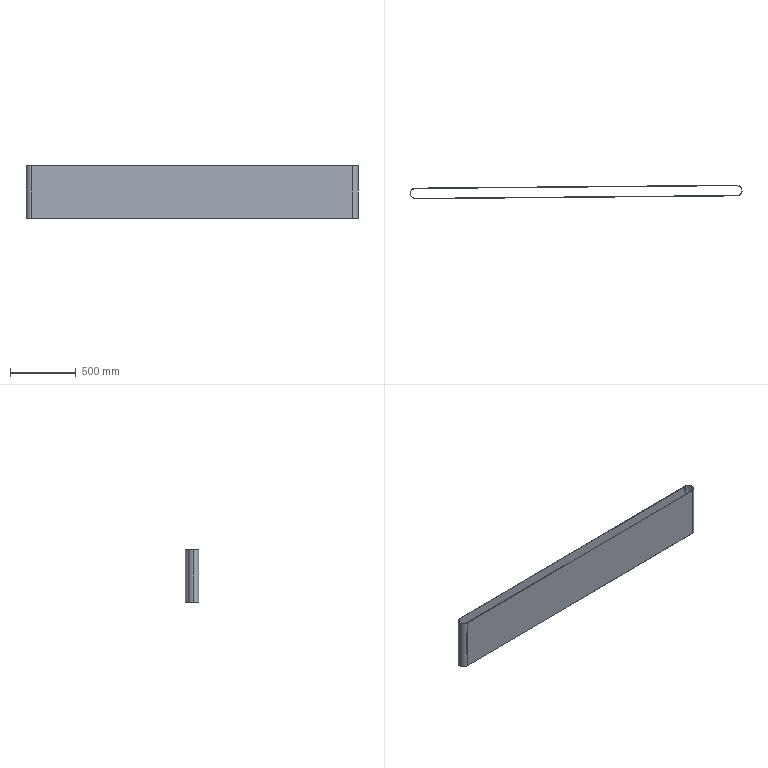Part | STEP file | Flat conveyor mechanism-strip | 1 solid | 18 faces | box 2534 x 103.36 x 400 mm | volume 5769946 mm3 | plane 12 | cylinder 6 | commonest cylinder face diameters 75.388 x3 80.988 x3
STEP:
#1=CARTESIAN_POINT('',(-1278.165,-120.803,200.));
#2=VERTEX_POINT('',#1);
#3=CARTESIAN_POINT('',(-1240.815,-83.11,200.));
#4=VERTEX_POINT('',#3);
#5=CARTESIAN_POINT('',(-1240.471,-120.803,200.));
#6=DIRECTION('',(0.,0.,-1.));
#7=DIRECTION('',(0.00912,-1.,0.));
#8=AXIS2_PLACEMENT_3D('',#5,#6,#7);
#9=CIRCLE('',#8,37.694);
#10=EDGE_CURVE('',#2,#4,#9,.T.);
#11=ORIENTED_EDGE('',*,*,#10,.F.);
#12=CARTESIAN_POINT('',(-1278.165,-120.803,-200.));
#13=VERTEX_POINT('',#12);
#14=CARTESIAN_POINT('',(-1278.165,-120.803,0.));
#15=DIRECTION('',(0.,0.,-1.));
#16=VECTOR('',#15,1000.);
#17=LINE('',#14,#16);
#18=EDGE_CURVE('',#2,#13,#17,.T.);
#19=ORIENTED_EDGE('',*,*,#18,.T.);
#20=CARTESIAN_POINT('',(-1240.815,-83.11,-200.));
#21=VERTEX_POINT('',#20);
#22=CARTESIAN_POINT('',(-1240.471,-120.803,-200.));
#23=DIRECTION('',(0.,0.,-1.));
#24=DIRECTION('',(0.00912,-1.,0.));
#25=AXIS2_PLACEMENT_3D('',#22,#23,#24);
#26=CIRCLE('',#25,37.694);
#27=EDGE_CURVE('',#13,#21,#26,.T.);
#28=ORIENTED_EDGE('',*,*,#27,.T.);
#29=CARTESIAN_POINT('',(-1240.815,-83.11,200.));
#30=DIRECTION('',(0.,0.,-1.));
#31=VECTOR('',#30,1000.);
#32=LINE('',#29,#31);
#33=EDGE_CURVE('',#4,#21,#32,.T.);
#34=ORIENTED_EDGE('',*,*,#33,.F.);
#35=EDGE_LOOP('',(#11,#19,#28,#34));
#36=FACE_OUTER_BOUND('',#35,.T.);
#37=CARTESIAN_POINT('',(-1240.471,-120.803,0.));
#38=DIRECTION('',(0.,0.,-1.));
#39=DIRECTION('',(-1.,0.,0.));
#40=AXIS2_PLACEMENT_3D('',#37,#38,#39);
#41=CYLINDRICAL_SURFACE('',#40,37.694);
#42=ADVANCED_FACE('',(#36),#41,.F.);
#43=CARTESIAN_POINT('',(-1240.101,-161.295,200.));
#44=VERTEX_POINT('',#43);
#45=CARTESIAN_POINT('',(-1280.965,-120.803,200.));
#46=VERTEX_POINT('',#45);
#47=CARTESIAN_POINT('',(-1240.471,-120.803,200.));
#48=DIRECTION('',(0.,0.,-1.));
#49=DIRECTION('',(0.00912,-1.,0.));
#50=AXIS2_PLACEMENT_3D('',#47,#48,#49);
#51=CIRCLE('',#50,40.494);
#52=EDGE_CURVE('',#44,#46,#51,.T.);
#53=ORIENTED_EDGE('',*,*,#52,.T.);
#54=CARTESIAN_POINT('',(-1280.965,-120.803,-200.));
#55=VERTEX_POINT('',#54);
#56=CARTESIAN_POINT('',(-1280.965,-120.803,0.));
#57=DIRECTION('',(0.,0.,-1.));
#58=VECTOR('',#57,1000.);
#59=LINE('',#56,#58);
#60=EDGE_CURVE('',#46,#55,#59,.T.);
#61=ORIENTED_EDGE('',*,*,#60,.T.);
#62=CARTESIAN_POINT('',(-1240.101,-161.295,-200.));
#63=VERTEX_POINT('',#62);
#64=CARTESIAN_POINT('',(-1240.471,-120.803,-200.));
#65=DIRECTION('',(0.,0.,-1.));
#66=DIRECTION('',(0.00912,-1.,0.));
#67=AXIS2_PLACEMENT_3D('',#64,#65,#66);
#68=CIRCLE('',#67,40.494);
#69=EDGE_CURVE('',#63,#55,#68,.T.);
#70=ORIENTED_EDGE('',*,*,#69,.F.);
#71=CARTESIAN_POINT('',(-1240.101,-161.295,200.));
#72=DIRECTION('',(0.,0.,1.));
#73=VECTOR('',#72,1000.);
#74=LINE('',#71,#73);
#75=EDGE_CURVE('',#63,#44,#74,.T.);
#76=ORIENTED_EDGE('',*,*,#75,.T.);
#77=EDGE_LOOP('',(#53,#61,#70,#76));
#78=FACE_OUTER_BOUND('',#77,.T.);
#79=CARTESIAN_POINT('',(-1240.471,-120.803,0.));
#80=DIRECTION('',(0.,0.,-1.));
#81=DIRECTION('',(-1.,0.,0.));
#82=AXIS2_PLACEMENT_3D('',#79,#80,#81);
#83=CYLINDRICAL_SURFACE('',#82,40.494);
#84=ADVANCED_FACE('',(#78),#83,.T.);
#85=CARTESIAN_POINT('',(-1240.84,-80.311,-200.));
#86=VERTEX_POINT('',#85);
#87=CARTESIAN_POINT('',(1212.109,-57.938,-200.));
#88=VERTEX_POINT('',#87);
#89=CARTESIAN_POINT('',(-1240.84,-80.311,-200.));
#90=DIRECTION('',(1.,0.00912,0.));
#91=VECTOR('',#90,1000.);
#92=LINE('',#89,#91);
#93=EDGE_CURVE('',#86,#88,#92,.T.);
#94=ORIENTED_EDGE('',*,*,#93,.F.);
#95=CARTESIAN_POINT('',(-1240.84,-80.311,200.));
#96=VERTEX_POINT('',#95);
#97=CARTESIAN_POINT('',(-1240.84,-80.311,200.));
#98=DIRECTION('',(0.,0.,1.));
#99=VECTOR('',#98,1000.);
#100=LINE('',#97,#99);
#101=EDGE_CURVE('',#86,#96,#100,.T.);
#102=ORIENTED_EDGE('',*,*,#101,.T.);
#103=CARTESIAN_POINT('',(1212.109,-57.938,200.));
#104=VERTEX_POINT('',#103);
#105=CARTESIAN_POINT('',(-1240.84,-80.311,200.));
#106=DIRECTION('',(1.,0.00912,0.));
#107=VECTOR('',#106,1000.);
#108=LINE('',#105,#107);
#109=EDGE_CURVE('',#96,#104,#108,.T.);
#110=ORIENTED_EDGE('',*,*,#109,.T.);
#111=CARTESIAN_POINT('',(1212.109,-57.938,200.));
#112=DIRECTION('',(0.,0.,1.));
#113=VECTOR('',#112,1000.);
#114=LINE('',#111,#113);
#115=EDGE_CURVE('',#88,#104,#114,.T.);
#116=ORIENTED_EDGE('',*,*,#115,.F.);
#117=EDGE_LOOP('',(#94,#102,#110,#116));
#118=FACE_OUTER_BOUND('',#117,.T.);
#119=CARTESIAN_POINT('',(-1240.84,-80.311,200.));
#120=DIRECTION('',(-0.00912,1.,0.));
#121=DIRECTION('',(-1.,-0.00912,0.));
#122=AXIS2_PLACEMENT_3D('',#119,#120,#121);
#123=PLANE('',#122);
#124=ADVANCED_FACE('',(#118),#123,.T.);
#125=CARTESIAN_POINT('',(1212.134,-60.738,-200.));
#126=VERTEX_POINT('',#125);
#127=CARTESIAN_POINT('',(-1240.815,-83.11,-200.));
#128=DIRECTION('',(1.,0.00912,0.));
#129=VECTOR('',#128,1000.);
#130=LINE('',#127,#129);
#131=EDGE_CURVE('',#21,#126,#130,.T.);
#132=ORIENTED_EDGE('',*,*,#131,.F.);
#133=CARTESIAN_POINT('',(-1240.84,-80.311,-200.));
#134=DIRECTION('',(-0.00912,1.,0.));
#135=VECTOR('',#134,1000.);
#136=LINE('',#133,#135);
#137=EDGE_CURVE('',#21,#86,#136,.T.);
#138=ORIENTED_EDGE('',*,*,#137,.T.);
#139=ORIENTED_EDGE('',*,*,#93,.T.);
#140=CARTESIAN_POINT('',(1212.109,-57.938,-200.));
#141=DIRECTION('',(-0.00912,1.,0.));
#142=VECTOR('',#141,1000.);
#143=LINE('',#140,#142);
#144=EDGE_CURVE('',#126,#88,#143,.T.);
#145=ORIENTED_EDGE('',*,*,#144,.F.);
#146=EDGE_LOOP('',(#132,#138,#139,#145));
#147=FACE_OUTER_BOUND('',#146,.T.);
#148=CARTESIAN_POINT('',(-1240.84,-80.311,-200.));
#149=DIRECTION('',(0.,0.,-1.));
#150=DIRECTION('',(-1.,0.,0.));
#151=AXIS2_PLACEMENT_3D('',#148,#149,#150);
#152=PLANE('',#151);
#153=ADVANCED_FACE('',(#147),#152,.T.);
#154=CARTESIAN_POINT('',(1212.134,-60.738,200.));
#155=VERTEX_POINT('',#154);
#156=CARTESIAN_POINT('',(-1240.815,-83.11,200.));
#157=DIRECTION('',(1.,0.00912,0.));
#158=VECTOR('',#157,1000.);
#159=LINE('',#156,#158);
#160=EDGE_CURVE('',#4,#155,#159,.T.);
#161=ORIENTED_EDGE('',*,*,#160,.F.);
#162=ORIENTED_EDGE('',*,*,#33,.T.);
#163=ORIENTED_EDGE('',*,*,#131,.T.);
#164=CARTESIAN_POINT('',(1212.134,-60.738,200.));
#165=DIRECTION('',(0.,0.,-1.));
#166=VECTOR('',#165,1000.);
#167=LINE('',#164,#166);
#168=EDGE_CURVE('',#155,#126,#167,.T.);
#169=ORIENTED_EDGE('',*,*,#168,.F.);
#170=EDGE_LOOP('',(#161,#162,#163,#169));
#171=FACE_OUTER_BOUND('',#170,.T.);
#172=CARTESIAN_POINT('',(-1240.815,-83.11,200.));
#173=DIRECTION('',(0.00912,-1.,0.));
#174=DIRECTION('',(1.,0.00912,0.));
#175=AXIS2_PLACEMENT_3D('',#172,#173,#174);
#176=PLANE('',#175);
#177=ADVANCED_FACE('',(#171),#176,.T.);
#178=ORIENTED_EDGE('',*,*,#60,.F.);
#179=CARTESIAN_POINT('',(-1240.471,-120.803,200.));
#180=DIRECTION('',(0.,0.,-1.));
#181=DIRECTION('',(0.00912,-1.,0.));
#182=AXIS2_PLACEMENT_3D('',#179,#180,#181);
#183=CIRCLE('',#182,40.494);
#184=EDGE_CURVE('',#46,#96,#183,.T.);
#185=ORIENTED_EDGE('',*,*,#184,.T.);
#186=ORIENTED_EDGE('',*,*,#101,.F.);
#187=CARTESIAN_POINT('',(-1240.471,-120.803,-200.));
#188=DIRECTION('',(0.,0.,-1.));
#189=DIRECTION('',(0.00912,-1.,0.));
#190=AXIS2_PLACEMENT_3D('',#187,#188,#189);
#191=CIRCLE('',#190,40.494);
#192=EDGE_CURVE('',#55,#86,#191,.T.);
#193=ORIENTED_EDGE('',*,*,#192,.F.);
#194=EDGE_LOOP('',(#178,#185,#186,#193));
#195=FACE_OUTER_BOUND('',#194,.T.);
#196=CARTESIAN_POINT('',(-1240.471,-120.803,0.));
#197=DIRECTION('',(0.,0.,-1.));
#198=DIRECTION('',(-1.,0.,0.));
#199=AXIS2_PLACEMENT_3D('',#196,#197,#198);
#200=CYLINDRICAL_SURFACE('',#199,40.494);
#201=ADVANCED_FACE('',(#195),#200,.T.);
#202=ORIENTED_EDGE('',*,*,#69,.T.);
#203=ORIENTED_EDGE('',*,*,#192,.T.);
#204=ORIENTED_EDGE('',*,*,#137,.F.);
#205=ORIENTED_EDGE('',*,*,#27,.F.);
#206=CARTESIAN_POINT('',(-1240.127,-158.495,-200.));
#207=VERTEX_POINT('',#206);
#208=CARTESIAN_POINT('',(-1240.471,-120.803,-200.));
#209=DIRECTION('',(0.,0.,-1.));
#210=DIRECTION('',(0.00912,-1.,0.));
#211=AXIS2_PLACEMENT_3D('',#208,#209,#210);
#212=CIRCLE('',#211,37.694);
#213=EDGE_CURVE('',#207,#13,#212,.T.);
#214=ORIENTED_EDGE('',*,*,#213,.F.);
#215=CARTESIAN_POINT('',(-1240.101,-161.295,-200.));
#216=DIRECTION('',(0.00912,-1.,0.));
#217=VECTOR('',#216,1000.);
#218=LINE('',#215,#217);
#219=EDGE_CURVE('',#207,#63,#218,.T.);
#220=ORIENTED_EDGE('',*,*,#219,.T.);
#221=EDGE_LOOP('',(#202,#203,#204,#205,#214,#220));
#222=FACE_OUTER_BOUND('',#221,.T.);
#223=CARTESIAN_POINT('',(-1240.101,-161.295,-200.));
#224=DIRECTION('',(0.,0.,-1.));
#225=DIRECTION('',(-1.,0.,0.));
#226=AXIS2_PLACEMENT_3D('',#223,#224,#225);
#227=PLANE('',#226);
#228=ADVANCED_FACE('',(#222),#227,.T.);
#229=ORIENTED_EDGE('',*,*,#18,.F.);
#230=CARTESIAN_POINT('',(-1240.127,-158.495,200.));
#231=VERTEX_POINT('',#230);
#232=CARTESIAN_POINT('',(-1240.471,-120.803,200.));
#233=DIRECTION('',(0.,0.,-1.));
#234=DIRECTION('',(0.00912,-1.,0.));
#235=AXIS2_PLACEMENT_3D('',#232,#233,#234);
#236=CIRCLE('',#235,37.694);
#237=EDGE_CURVE('',#231,#2,#236,.T.);
#238=ORIENTED_EDGE('',*,*,#237,.F.);
#239=CARTESIAN_POINT('',(-1240.127,-158.495,200.));
#240=DIRECTION('',(0.,0.,-1.));
#241=VECTOR('',#240,1000.);
#242=LINE('',#239,#241);
#243=EDGE_CURVE('',#231,#207,#242,.T.);
#244=ORIENTED_EDGE('',*,*,#243,.T.);
#245=ORIENTED_EDGE('',*,*,#213,.T.);
#246=EDGE_LOOP('',(#229,#238,#244,#245));
#247=FACE_OUTER_BOUND('',#246,.T.);
#248=CARTESIAN_POINT('',(-1240.471,-120.803,0.));
#249=DIRECTION('',(0.,0.,-1.));
#250=DIRECTION('',(-1.,0.,0.));
#251=AXIS2_PLACEMENT_3D('',#248,#249,#250);
#252=CYLINDRICAL_SURFACE('',#251,37.694);
#253=ADVANCED_FACE('',(#247),#252,.F.);
#254=ORIENTED_EDGE('',*,*,#237,.T.);
#255=ORIENTED_EDGE('',*,*,#10,.T.);
#256=CARTESIAN_POINT('',(-1240.84,-80.311,200.));
#257=DIRECTION('',(0.00912,-1.,0.));
#258=VECTOR('',#257,1000.);
#259=LINE('',#256,#258);
#260=EDGE_CURVE('',#96,#4,#259,.T.);
#261=ORIENTED_EDGE('',*,*,#260,.F.);
#262=ORIENTED_EDGE('',*,*,#184,.F.);
#263=ORIENTED_EDGE('',*,*,#52,.F.);
#264=CARTESIAN_POINT('',(-1240.101,-161.295,200.));
#265=DIRECTION('',(-0.00912,1.,0.));
#266=VECTOR('',#265,1000.);
#267=LINE('',#264,#266);
#268=EDGE_CURVE('',#44,#231,#267,.T.);
#269=ORIENTED_EDGE('',*,*,#268,.T.);
#270=EDGE_LOOP('',(#254,#255,#261,#262,#263,#269));
#271=FACE_OUTER_BOUND('',#270,.T.);
#272=CARTESIAN_POINT('',(-1240.101,-161.295,200.));
#273=DIRECTION('',(0.,0.,1.));
#274=DIRECTION('',(1.,0.,0.));
#275=AXIS2_PLACEMENT_3D('',#272,#273,#274);
#276=PLANE('',#275);
#277=ADVANCED_FACE('',(#271),#276,.T.);
#278=ORIENTED_EDGE('',*,*,#75,.F.);
#279=CARTESIAN_POINT('',(1212.847,-138.923,-200.));
#280=VERTEX_POINT('',#279);
#281=CARTESIAN_POINT('',(1212.847,-138.923,-200.));
#282=DIRECTION('',(-1.,-0.00912,0.));
#283=VECTOR('',#282,1000.);
#284=LINE('',#281,#283);
#285=EDGE_CURVE('',#280,#63,#284,.T.);
#286=ORIENTED_EDGE('',*,*,#285,.F.);
#287=CARTESIAN_POINT('',(1212.847,-138.923,200.));
#288=VERTEX_POINT('',#287);
#289=CARTESIAN_POINT('',(1212.847,-138.923,200.));
#290=DIRECTION('',(0.,0.,1.));
#291=VECTOR('',#290,1000.);
#292=LINE('',#289,#291);
#293=EDGE_CURVE('',#280,#288,#292,.T.);
#294=ORIENTED_EDGE('',*,*,#293,.T.);
#295=CARTESIAN_POINT('',(1212.847,-138.923,200.));
#296=DIRECTION('',(-1.,-0.00912,0.));
#297=VECTOR('',#296,1000.);
#298=LINE('',#295,#297);
#299=EDGE_CURVE('',#288,#44,#298,.T.);
#300=ORIENTED_EDGE('',*,*,#299,.T.);
#301=EDGE_LOOP('',(#278,#286,#294,#300));
#302=FACE_OUTER_BOUND('',#301,.T.);
#303=CARTESIAN_POINT('',(1212.847,-138.923,200.));
#304=DIRECTION('',(0.00912,-1.,0.));
#305=DIRECTION('',(1.,0.00912,0.));
#306=AXIS2_PLACEMENT_3D('',#303,#304,#305);
#307=PLANE('',#306);
#308=ADVANCED_FACE('',(#302),#307,.T.);
#309=ORIENTED_EDGE('',*,*,#285,.T.);
#310=ORIENTED_EDGE('',*,*,#219,.F.);
#311=CARTESIAN_POINT('',(1212.822,-136.123,-200.));
#312=VERTEX_POINT('',#311);
#313=CARTESIAN_POINT('',(1212.822,-136.123,-200.));
#314=DIRECTION('',(-1.,-0.00912,0.));
#315=VECTOR('',#314,1000.);
#316=LINE('',#313,#315);
#317=EDGE_CURVE('',#312,#207,#316,.T.);
#318=ORIENTED_EDGE('',*,*,#317,.F.);
#319=CARTESIAN_POINT('',(1212.847,-138.923,-200.));
#320=DIRECTION('',(0.00912,-1.,0.));
#321=VECTOR('',#320,1000.);
#322=LINE('',#319,#321);
#323=EDGE_CURVE('',#312,#280,#322,.T.);
#324=ORIENTED_EDGE('',*,*,#323,.T.);
#325=EDGE_LOOP('',(#309,#310,#318,#324));
#326=FACE_OUTER_BOUND('',#325,.T.);
#327=CARTESIAN_POINT('',(1212.847,-138.923,-200.));
#328=DIRECTION('',(0.,0.,-1.));
#329=DIRECTION('',(-1.,0.,0.));
#330=AXIS2_PLACEMENT_3D('',#327,#328,#329);
#331=PLANE('',#330);
#332=ADVANCED_FACE('',(#326),#331,.T.);
#333=ORIENTED_EDGE('',*,*,#317,.T.);
#334=ORIENTED_EDGE('',*,*,#243,.F.);
#335=CARTESIAN_POINT('',(1212.822,-136.123,200.));
#336=VERTEX_POINT('',#335);
#337=CARTESIAN_POINT('',(1212.822,-136.123,200.));
#338=DIRECTION('',(-1.,-0.00912,0.));
#339=VECTOR('',#338,1000.);
#340=LINE('',#337,#339);
#341=EDGE_CURVE('',#336,#231,#340,.T.);
#342=ORIENTED_EDGE('',*,*,#341,.F.);
#343=CARTESIAN_POINT('',(1212.822,-136.123,200.));
#344=DIRECTION('',(0.,0.,-1.));
#345=VECTOR('',#344,1000.);
#346=LINE('',#343,#345);
#347=EDGE_CURVE('',#336,#312,#346,.T.);
#348=ORIENTED_EDGE('',*,*,#347,.T.);
#349=EDGE_LOOP('',(#333,#334,#342,#348));
#350=FACE_OUTER_BOUND('',#349,.T.);
#351=CARTESIAN_POINT('',(1212.822,-136.123,200.));
#352=DIRECTION('',(-0.00912,1.,0.));
#353=DIRECTION('',(-1.,-0.00912,0.));
#354=AXIS2_PLACEMENT_3D('',#351,#352,#353);
#355=PLANE('',#354);
#356=ADVANCED_FACE('',(#350),#355,.T.);
#357=ORIENTED_EDGE('',*,*,#341,.T.);
#358=ORIENTED_EDGE('',*,*,#268,.F.);
#359=ORIENTED_EDGE('',*,*,#299,.F.);
#360=CARTESIAN_POINT('',(1212.847,-138.923,200.));
#361=DIRECTION('',(-0.00912,1.,0.));
#362=VECTOR('',#361,1000.);
#363=LINE('',#360,#362);
#364=EDGE_CURVE('',#288,#336,#363,.T.);
#365=ORIENTED_EDGE('',*,*,#364,.T.);
#366=EDGE_LOOP('',(#357,#358,#359,#365));
#367=FACE_OUTER_BOUND('',#366,.T.);
#368=CARTESIAN_POINT('',(1212.847,-138.923,200.));
#369=DIRECTION('',(0.,0.,1.));
#370=DIRECTION('',(1.,0.,0.));
#371=AXIS2_PLACEMENT_3D('',#368,#369,#370);
#372=PLANE('',#371);
#373=ADVANCED_FACE('',(#367),#372,.T.);
#374=ORIENTED_EDGE('',*,*,#293,.F.);
#375=CARTESIAN_POINT('',(1212.478,-98.431,-200.));
#376=DIRECTION('',(0.,0.,-1.));
#377=DIRECTION('',(-0.00912,1.,0.));
#378=AXIS2_PLACEMENT_3D('',#375,#376,#377);
#379=CIRCLE('',#378,40.494);
#380=EDGE_CURVE('',#88,#280,#379,.T.);
#381=ORIENTED_EDGE('',*,*,#380,.F.);
#382=ORIENTED_EDGE('',*,*,#115,.T.);
#383=CARTESIAN_POINT('',(1212.478,-98.431,200.));
#384=DIRECTION('',(0.,0.,-1.));
#385=DIRECTION('',(-0.00912,1.,0.));
#386=AXIS2_PLACEMENT_3D('',#383,#384,#385);
#387=CIRCLE('',#386,40.494);
#388=EDGE_CURVE('',#104,#288,#387,.T.);
#389=ORIENTED_EDGE('',*,*,#388,.T.);
#390=EDGE_LOOP('',(#374,#381,#382,#389));
#391=FACE_OUTER_BOUND('',#390,.T.);
#392=CARTESIAN_POINT('',(1212.478,-98.431,0.));
#393=DIRECTION('',(0.,0.,-1.));
#394=DIRECTION('',(-1.,0.,0.));
#395=AXIS2_PLACEMENT_3D('',#392,#393,#394);
#396=CYLINDRICAL_SURFACE('',#395,40.494);
#397=ADVANCED_FACE('',(#391),#396,.T.);
#398=ORIENTED_EDGE('',*,*,#380,.T.);
#399=ORIENTED_EDGE('',*,*,#323,.F.);
#400=CARTESIAN_POINT('',(1212.478,-98.431,-200.));
#401=DIRECTION('',(0.,0.,-1.));
#402=DIRECTION('',(-0.00912,1.,0.));
#403=AXIS2_PLACEMENT_3D('',#400,#401,#402);
#404=CIRCLE('',#403,37.694);
#405=EDGE_CURVE('',#126,#312,#404,.T.);
#406=ORIENTED_EDGE('',*,*,#405,.F.);
#407=ORIENTED_EDGE('',*,*,#144,.T.);
#408=EDGE_LOOP('',(#398,#399,#406,#407));
#409=FACE_OUTER_BOUND('',#408,.T.);
#410=CARTESIAN_POINT('',(1212.109,-57.938,-200.));
#411=DIRECTION('',(0.,0.,-1.));
#412=DIRECTION('',(-1.,0.,0.));
#413=AXIS2_PLACEMENT_3D('',#410,#411,#412);
#414=PLANE('',#413);
#415=ADVANCED_FACE('',(#409),#414,.T.);
#416=ORIENTED_EDGE('',*,*,#405,.T.);
#417=ORIENTED_EDGE('',*,*,#347,.F.);
#418=CARTESIAN_POINT('',(1212.478,-98.431,200.));
#419=DIRECTION('',(0.,0.,-1.));
#420=DIRECTION('',(-0.00912,1.,0.));
#421=AXIS2_PLACEMENT_3D('',#418,#419,#420);
#422=CIRCLE('',#421,37.694);
#423=EDGE_CURVE('',#155,#336,#422,.T.);
#424=ORIENTED_EDGE('',*,*,#423,.F.);
#425=ORIENTED_EDGE('',*,*,#168,.T.);
#426=EDGE_LOOP('',(#416,#417,#424,#425));
#427=FACE_OUTER_BOUND('',#426,.T.);
#428=CARTESIAN_POINT('',(1212.478,-98.431,0.));
#429=DIRECTION('',(0.,0.,-1.));
#430=DIRECTION('',(-1.,0.,0.));
#431=AXIS2_PLACEMENT_3D('',#428,#429,#430);
#432=CYLINDRICAL_SURFACE('',#431,37.694);
#433=ADVANCED_FACE('',(#427),#432,.F.);
#434=ORIENTED_EDGE('',*,*,#423,.T.);
#435=ORIENTED_EDGE('',*,*,#364,.F.);
#436=ORIENTED_EDGE('',*,*,#388,.F.);
#437=CARTESIAN_POINT('',(1212.109,-57.938,200.));
#438=DIRECTION('',(0.00912,-1.,0.));
#439=VECTOR('',#438,1000.);
#440=LINE('',#437,#439);
#441=EDGE_CURVE('',#104,#155,#440,.T.);
#442=ORIENTED_EDGE('',*,*,#441,.T.);
#443=EDGE_LOOP('',(#434,#435,#436,#442));
#444=FACE_OUTER_BOUND('',#443,.T.);
#445=CARTESIAN_POINT('',(1212.109,-57.938,200.));
#446=DIRECTION('',(0.,0.,1.));
#447=DIRECTION('',(1.,0.,0.));
#448=AXIS2_PLACEMENT_3D('',#445,#446,#447);
#449=PLANE('',#448);
#450=ADVANCED_FACE('',(#444),#449,.T.);
#451=ORIENTED_EDGE('',*,*,#260,.T.);
#452=ORIENTED_EDGE('',*,*,#160,.T.);
#453=ORIENTED_EDGE('',*,*,#441,.F.);
#454=ORIENTED_EDGE('',*,*,#109,.F.);
#455=EDGE_LOOP('',(#451,#452,#453,#454));
#456=FACE_OUTER_BOUND('',#455,.T.);
#457=CARTESIAN_POINT('',(-1240.84,-80.311,200.));
#458=DIRECTION('',(0.,0.,1.));
#459=DIRECTION('',(1.,0.,0.));
#460=AXIS2_PLACEMENT_3D('',#457,#458,#459);
#461=PLANE('',#460);
#462=ADVANCED_FACE('',(#456),#461,.T.);
#463=CLOSED_SHELL('',(#42,#84,#124,#153,#177,#201,#228,#253,#277,#308,#332,#356,#373,#397,#415,#433,#450,#462));
#464=MANIFOLD_SOLID_BREP('',#463);
#465=CARTESIAN_POINT('',(0.,0.,0.));
#466=DIRECTION('',(0.,0.,1.));
#467=DIRECTION('',(1.,0.,0.));
#468=AXIS2_PLACEMENT_3D('',#465,#466,#467);
#469=(LENGTH_UNIT()NAMED_UNIT(*)SI_UNIT(.MILLI.,.METRE.));
#470=UNCERTAINTY_MEASURE_WITH_UNIT(LENGTH_MEASURE(0.00001),#469,'','');
#471=(NAMED_UNIT(*)PLANE_ANGLE_UNIT()SI_UNIT($,.RADIAN.));
#472=(NAMED_UNIT(*)SI_UNIT($,.STERADIAN.)SOLID_ANGLE_UNIT());
#473=(GEOMETRIC_REPRESENTATION_CONTEXT(3)GLOBAL_UNCERTAINTY_ASSIGNED_CONTEXT((#470))GLOBAL_UNIT_ASSIGNED_CONTEXT((#469,#471,#472))REPRESENTATION_CONTEXT('',''));
#474=ADVANCED_BREP_SHAPE_REPRESENTATION('',(#464,#468),#473);